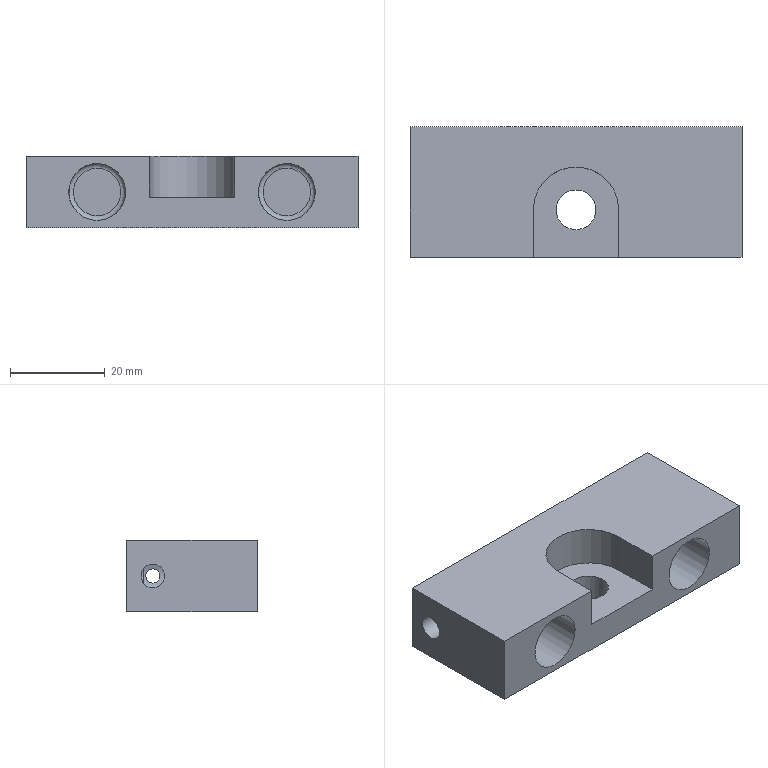NC program | NX | posted with a generic post | part box 70 x 27.5 x 15 mm
Lines 28 to 859 of 3781:
(PLANAR_MILL_8 , TOOL : D8-25-D8-60-3T-ROUGH)
N48 T03 M6
N50 G54
N52 G17 G0 G90 X-21.509 Y1.151 B0. C0. S2500 M3
N54 G43 Z20. H3
N56 Z1. B-180. C-180.
N58 G94 G1 X-21.592 Y1.043 Z0.993 F600.
N60 X-21.699 Y0.857 Z0.982
N62 X-21.809 Y0.59 Z0.966
N64 X-21.878 Y0.308 Z0.951
N66 X-21.903 Y0.019 Z0.936
N68 X-21.884 Y-0.27 Z0.921
N70 X-21.821 Y-0.553 Z0.906
N72 X-21.716 Y-0.823 Z0.891
N74 X-21.571 Y-1.074 Z0.875
N76 X-21.389 Y-1.3 Z0.86
N78 X-21.176 Y-1.496 Z0.845
N80 X-20.935 Y-1.658 Z0.83
N82 X-20.672 Y-1.78 Z0.815
N84 X-20.394 Y-1.862 Z0.799
N86 X-20.107 Y-1.9 Z0.784
N88 X-19.893 Z0.773
N90 X-19.606 Y-1.862 Z0.758
N92 X-19.328 Y-1.78 Z0.743
N94 X-19.065 Y-1.658 Z0.727
N96 X-18.824 Y-1.496 Z0.712
N98 X-18.611 Y-1.3 Z0.697
N100 X-18.429 Y-1.074 Z0.682
N102 X-18.284 Y-0.823 Z0.667
N104 X-18.179 Y-0.553 Z0.651
N106 X-18.116 Y-0.27 Z0.636
N108 X-18.097 Y0.019 Z0.621
N110 X-18.122 Y0.308 Z0.606
N112 X-18.191 Y0.59 Z0.591
N114 X-18.301 Y0.857 Z0.575
N116 X-18.408 Y1.043 Z0.564
N118 X-18.589 Y1.277 Z0.549
N120 X-18.804 Y1.48 Z0.533
N122 X-19.049 Y1.648 Z0.518
N124 X-19.316 Y1.776 Z0.502
N126 X-19.6 Y1.86 Z0.487
N128 X-19.893 Y1.9 Z0.471
N130 X-20.107 Z0.46
N132 X-20.4 Y1.86 Z0.444
N134 X-20.684 Y1.776 Z0.429
N136 X-20.952 Y1.648 Z0.413
N138 X-21.196 Y1.48 Z0.398
N140 X-21.411 Y1.277 Z0.382
N142 X-21.592 Y1.043 Z0.367
N144 X-21.699 Y0.857 Z0.356
N146 X-21.809 Y0.59 Z0.34
N148 X-21.878 Y0.308 Z0.325
N150 X-21.903 Y0.019 Z0.31
N152 X-21.884 Y-0.27 Z0.295
N154 X-21.821 Y-0.553 Z0.28
N156 X-21.716 Y-0.823 Z0.264
N158 X-21.571 Y-1.074 Z0.249
N160 X-21.389 Y-1.3 Z0.234
N162 X-21.176 Y-1.496 Z0.219
N164 X-20.935 Y-1.658 Z0.204
N166 X-20.672 Y-1.78 Z0.189
N168 X-20.394 Y-1.862 Z0.173
N170 X-20.107 Y-1.9 Z0.158
N172 X-19.893 Z0.147
N174 X-19.606 Y-1.862 Z0.132
N176 X-19.328 Y-1.78 Z0.117
N178 X-19.065 Y-1.658 Z0.101
N180 X-18.824 Y-1.496 Z0.086
N182 X-18.611 Y-1.3 Z0.071
N184 X-18.429 Y-1.074 Z0.056
N186 X-18.284 Y-0.823 Z0.041
N188 X-18.179 Y-0.553 Z0.025
N190 X-18.116 Y-0.27 Z0.01
N192 X-18.097 Y0.019 Z-0.005
N194 X-18.122 Y0.308 Z-0.02
N196 X-18.191 Y0.59 Z-0.035
N198 X-18.301 Y0.857 Z-0.051
N200 X-18.408 Y1.043 Z-0.062
N202 X-18.589 Y1.277 Z-0.077
N204 X-18.804 Y1.48 Z-0.093
N206 X-19.049 Y1.648 Z-0.108
N208 X-19.316 Y1.776 Z-0.124
N210 X-19.6 Y1.86 Z-0.139
N212 X-19.893 Y1.9 Z-0.155
N214 X-20.107 Z-0.166
N216 X-20.4 Y1.86 Z-0.182
N218 X-20.684 Y1.776 Z-0.197
N220 X-20.952 Y1.648 Z-0.213
N222 X-21.196 Y1.48 Z-0.228
N224 X-21.411 Y1.277 Z-0.244
N226 X-21.592 Y1.043 Z-0.259
N228 X-21.699 Y0.857 Z-0.27
N230 X-21.809 Y0.59 Z-0.286
N232 X-21.878 Y0.308 Z-0.301
N234 X-21.903 Y0.019 Z-0.316
N236 X-21.884 Y-0.27 Z-0.331
N238 X-21.821 Y-0.553 Z-0.346
N240 X-21.716 Y-0.823 Z-0.362
N242 X-21.571 Y-1.074 Z-0.377
N244 X-21.389 Y-1.3 Z-0.392
N246 X-21.176 Y-1.496 Z-0.407
N248 X-20.935 Y-1.658 Z-0.422
N250 X-20.672 Y-1.78 Z-0.438
N252 X-20.394 Y-1.862 Z-0.453
N254 X-20.107 Y-1.9 Z-0.468
N256 X-19.893 Z-0.479
N258 X-19.606 Y-1.862 Z-0.494
N260 X-19.328 Y-1.78 Z-0.509
N262 X-19.065 Y-1.658 Z-0.525
N264 X-18.824 Y-1.496 Z-0.54
N266 X-18.611 Y-1.3 Z-0.555
N268 X-18.429 Y-1.074 Z-0.57
N270 X-18.284 Y-0.823 Z-0.585
N272 X-18.179 Y-0.553 Z-0.601
N274 X-18.116 Y-0.27 Z-0.616
N276 X-18.097 Y0.019 Z-0.631
N278 X-18.122 Y0.308 Z-0.646
N280 X-18.191 Y0.59 Z-0.661
N282 X-18.301 Y0.857 Z-0.677
N284 X-18.408 Y1.043 Z-0.688
N286 X-18.589 Y1.277 Z-0.703
N288 X-18.804 Y1.48 Z-0.719
N290 X-19.049 Y1.648 Z-0.734
N292 X-19.316 Y1.776 Z-0.75
N294 X-19.6 Y1.86 Z-0.765
N296 X-19.893 Y1.9 Z-0.781
N298 X-20.107 Z-0.792
N300 X-20.4 Y1.86 Z-0.808
N302 X-20.684 Y1.776 Z-0.823
N304 X-20.952 Y1.648 Z-0.839
N306 X-21.196 Y1.48 Z-0.854
N308 X-21.411 Y1.277 Z-0.87
N310 X-21.592 Y1.043 Z-0.885
N312 X-21.699 Y0.857 Z-0.896
N314 X-21.809 Y0.59 Z-0.912
N316 X-21.878 Y0.308 Z-0.927
N318 X-21.903 Y0.019 Z-0.942
N320 X-21.884 Y-0.27 Z-0.957
N322 X-21.821 Y-0.553 Z-0.972
N324 X-21.716 Y-0.823 Z-0.988
N326 X-21.571 Y-1.074 Z-1.003
N328 X-21.389 Y-1.3 Z-1.018
N330 X-21.176 Y-1.496 Z-1.033
N332 X-20.935 Y-1.658 Z-1.048
N334 X-20.672 Y-1.78 Z-1.064
N336 X-20.394 Y-1.862 Z-1.079
N338 X-20.107 Y-1.9 Z-1.094
N340 X-19.893 Z-1.105
N342 X-19.606 Y-1.862 Z-1.12
N344 X-19.328 Y-1.78 Z-1.136
N346 X-19.065 Y-1.658 Z-1.151
N348 X-18.824 Y-1.496 Z-1.166
N350 X-18.611 Y-1.3 Z-1.181
N352 X-18.429 Y-1.074 Z-1.196
N354 X-18.284 Y-0.823 Z-1.211
N356 X-18.179 Y-0.553 Z-1.227
N358 X-18.116 Y-0.27 Z-1.242
N360 X-18.097 Y0.019 Z-1.257
N362 X-18.122 Y0.308 Z-1.272
N364 X-18.191 Y0.59 Z-1.287
N366 X-18.301 Y0.857 Z-1.303
N368 X-18.408 Y1.043 Z-1.314
N370 X-18.589 Y1.277 Z-1.329
N372 X-18.804 Y1.48 Z-1.345
N374 X-19.049 Y1.648 Z-1.36
N376 X-19.316 Y1.776 Z-1.376
N378 X-19.6 Y1.86 Z-1.391
N380 X-19.893 Y1.9 Z-1.407
N382 X-20.107 Z-1.418
N384 X-20.4 Y1.86 Z-1.434
N386 X-20.684 Y1.776 Z-1.449
N388 X-20.952 Y1.648 Z-1.465
N390 X-21.196 Y1.48 Z-1.48
N392 X-21.411 Y1.277 Z-1.496
N394 X-21.592 Y1.043 Z-1.511
N396 X-21.699 Y0.857 Z-1.523
N398 X-21.809 Y0.59 Z-1.538
N400 X-21.878 Y0.308 Z-1.553
N402 X-21.903 Y0.019 Z-1.568
N404 X-21.884 Y-0.27 Z-1.583
N406 X-21.821 Y-0.553 Z-1.598
N408 X-21.716 Y-0.823 Z-1.614
N410 X-21.571 Y-1.074 Z-1.629
N412 X-21.389 Y-1.3 Z-1.644
N414 X-21.176 Y-1.496 Z-1.659
N416 X-20.935 Y-1.658 Z-1.674
N418 X-20.672 Y-1.78 Z-1.69
N420 X-20.394 Y-1.862 Z-1.705
N422 X-20.107 Y-1.9 Z-1.72
N424 X-19.893 Z-1.731
N426 X-19.606 Y-1.862 Z-1.746
N428 X-19.328 Y-1.78 Z-1.762
N430 X-19.065 Y-1.658 Z-1.777
N432 X-18.824 Y-1.496 Z-1.792
N434 X-18.611 Y-1.3 Z-1.807
N436 X-18.429 Y-1.074 Z-1.822
N438 X-18.284 Y-0.823 Z-1.838
N440 X-18.179 Y-0.553 Z-1.853
N442 X-18.116 Y-0.27 Z-1.868
N444 X-18.097 Y0.019 Z-1.883
N446 X-18.122 Y0.308 Z-1.898
N448 X-18.191 Y0.59 Z-1.913
N450 X-18.301 Y0.857 Z-1.929
N452 X-18.408 Y1.043 Z-1.94
N454 X-18.589 Y1.277 Z-1.955
N456 X-18.804 Y1.48 Z-1.971
N458 X-19.049 Y1.648 Z-1.986
N460 X-19.316 Y1.776 Z-2.002
N462 X-19.6 Y1.86 Z-2.017
N464 X-19.893 Y1.9 Z-2.033
N466 X-20.107 Z-2.044
N468 X-20.4 Y1.86 Z-2.06
N470 X-20.684 Y1.776 Z-2.075
N472 X-20.952 Y1.648 Z-2.091
N474 X-21.196 Y1.48 Z-2.106
N476 X-21.411 Y1.277 Z-2.122
N478 X-21.592 Y1.043 Z-2.137
N480 X-21.699 Y0.857 Z-2.149
N482 X-21.809 Y0.59 Z-2.164
N484 X-21.878 Y0.308 Z-2.179
N486 X-21.903 Y0.019 Z-2.194
N488 X-21.884 Y-0.27 Z-2.209
N490 X-21.821 Y-0.553 Z-2.225
N492 X-21.716 Y-0.823 Z-2.24
N494 X-21.571 Y-1.074 Z-2.255
N496 X-21.389 Y-1.3 Z-2.27
N498 X-21.176 Y-1.496 Z-2.285
N500 X-20.935 Y-1.658 Z-2.3
N502 X-20.672 Y-1.78 Z-2.316
N504 X-20.394 Y-1.862 Z-2.331
N506 X-20.107 Y-1.9 Z-2.346
N508 X-19.893 Z-2.357
N510 X-19.606 Y-1.862 Z-2.372
N512 X-19.328 Y-1.78 Z-2.388
N514 X-19.065 Y-1.658 Z-2.403
N516 X-18.824 Y-1.496 Z-2.418
N518 X-18.611 Y-1.3 Z-2.433
N520 X-18.429 Y-1.074 Z-2.448
N522 X-18.284 Y-0.823 Z-2.464
N524 X-18.179 Y-0.553 Z-2.479
N526 X-18.116 Y-0.27 Z-2.494
N528 X-18.097 Y0.019 Z-2.509
N530 X-18.122 Y0.308 Z-2.524
N532 X-18.191 Y0.59 Z-2.54
N534 X-18.301 Y0.857 Z-2.555
N536 X-18.408 Y1.043 Z-2.566
N538 X-18.589 Y1.277 Z-2.581
N540 X-18.804 Y1.48 Z-2.597
N542 X-19.049 Y1.648 Z-2.612
N544 X-19.316 Y1.776 Z-2.628
N546 X-19.6 Y1.86 Z-2.644
N548 X-19.893 Y1.9 Z-2.659
N550 X-20.107 Z-2.67
N552 X-20.4 Y1.86 Z-2.686
N554 X-20.684 Y1.776 Z-2.701
N556 X-20.952 Y1.648 Z-2.717
N558 X-21.196 Y1.48 Z-2.732
N560 X-21.411 Y1.277 Z-2.748
N562 X-21.592 Y1.043 Z-2.763
N564 X-21.699 Y0.857 Z-2.775
N566 X-21.809 Y0.59 Z-2.79
N568 X-21.878 Y0.308 Z-2.805
N570 X-21.903 Y0.019 Z-2.82
N572 X-21.884 Y-0.27 Z-2.835
N574 X-21.821 Y-0.553 Z-2.851
N576 X-21.716 Y-0.823 Z-2.866
N578 X-21.571 Y-1.074 Z-2.881
N580 X-21.389 Y-1.3 Z-2.896
N582 X-21.176 Y-1.496 Z-2.911
N584 X-20.935 Y-1.658 Z-2.926
N586 X-20.672 Y-1.78 Z-2.942
N588 X-20.394 Y-1.862 Z-2.957
N590 X-20.107 Y-1.9 Z-2.972
N592 X-19.893 Z-2.983
N594 X-19.606 Y-1.862 Z-2.998
N596 X-19.328 Y-1.78 Z-3.014
N598 X-19.065 Y-1.658 Z-3.029
N600 X-18.824 Y-1.496 Z-3.044
N602 X-18.611 Y-1.3 Z-3.059
N604 X-18.429 Y-1.074 Z-3.074
N606 X-18.284 Y-0.823 Z-3.09
N608 X-18.179 Y-0.553 Z-3.105
N610 X-18.116 Y-0.27 Z-3.12
N612 X-18.097 Y0.019 Z-3.135
N614 X-18.122 Y0.308 Z-3.15
N616 X-18.191 Y0.59 Z-3.166
N618 X-18.301 Y0.857 Z-3.181
N620 X-18.408 Y1.043 Z-3.192
N622 X-18.589 Y1.277 Z-3.207
N624 X-18.804 Y1.48 Z-3.223
N626 X-19.049 Y1.648 Z-3.239
N628 X-19.316 Y1.776 Z-3.254
N630 X-19.6 Y1.86 Z-3.27
N632 X-19.893 Y1.9 Z-3.285
N634 X-20.107 Z-3.296
N636 X-20.4 Y1.86 Z-3.312
N638 X-20.684 Y1.776 Z-3.327
N640 X-20.952 Y1.648 Z-3.343
N642 X-21.196 Y1.48 Z-3.358
N644 X-21.411 Y1.277 Z-3.374
N646 X-21.592 Y1.043 Z-3.389
N648 X-21.699 Y0.857 Z-3.401
N650 X-21.809 Y0.59 Z-3.416
N652 X-21.878 Y0.308 Z-3.431
N654 X-21.903 Y0.019 Z-3.446
N656 X-21.884 Y-0.27 Z-3.461
N658 X-21.821 Y-0.553 Z-3.477
N660 X-21.716 Y-0.823 Z-3.492
N662 X-21.571 Y-1.074 Z-3.507
N664 X-21.389 Y-1.3 Z-3.522
N666 X-21.176 Y-1.496 Z-3.537
N668 X-20.935 Y-1.658 Z-3.553
N670 X-20.672 Y-1.78 Z-3.568
N672 X-20.394 Y-1.862 Z-3.583
N674 X-20.107 Y-1.9 Z-3.598
N676 X-19.893 Z-3.609
N678 X-19.606 Y-1.862 Z-3.624
N680 X-19.328 Y-1.78 Z-3.64
N682 X-19.065 Y-1.658 Z-3.655
N684 X-18.824 Y-1.496 Z-3.67
N686 X-18.611 Y-1.3 Z-3.685
N688 X-18.429 Y-1.074 Z-3.7
N690 X-18.284 Y-0.823 Z-3.716
N692 X-18.179 Y-0.553 Z-3.731
N694 X-18.116 Y-0.27 Z-3.746
N696 X-18.097 Y0.019 Z-3.761
N698 X-18.122 Y0.308 Z-3.776
N700 X-18.191 Y0.59 Z-3.792
N702 X-18.301 Y0.857 Z-3.807
N704 X-18.408 Y1.043 Z-3.818
N706 X-18.589 Y1.277 Z-3.834
N708 X-18.804 Y1.48 Z-3.849
N710 X-19.049 Y1.648 Z-3.865
N712 X-19.316 Y1.776 Z-3.88
N714 X-19.6 Y1.86 Z-3.896
N716 X-19.893 Y1.9 Z-3.911
N718 X-20.107 Z-3.922
N720 X-20.4 Y1.86 Z-3.938
N722 X-20.684 Y1.776 Z-3.953
N724 X-20.952 Y1.648 Z-3.969
N726 X-21.196 Y1.48 Z-3.984
N728 X-21.411 Y1.277 Z-4.
N730 X-21.592 Y1.043 Z-4.015
N732 X-21.699 Y0.857 Z-4.027
N734 X-21.809 Y0.59 Z-4.042
N736 X-21.878 Y0.308 Z-4.057
N738 X-21.903 Y0.019 Z-4.072
N740 X-21.884 Y-0.27 Z-4.087
N742 X-21.821 Y-0.553 Z-4.103
N744 X-21.716 Y-0.823 Z-4.118
N746 X-21.571 Y-1.074 Z-4.133
N748 X-21.389 Y-1.3 Z-4.148
N750 X-21.176 Y-1.496 Z-4.163
N752 X-20.935 Y-1.658 Z-4.179
N754 X-20.672 Y-1.78 Z-4.194
N756 X-20.394 Y-1.862 Z-4.209
N758 X-20.107 Y-1.9 Z-4.224
N760 X-19.893 Z-4.235
N762 X-19.606 Y-1.862 Z-4.251
N764 X-19.328 Y-1.78 Z-4.266
N766 X-19.065 Y-1.658 Z-4.281
N768 X-18.824 Y-1.496 Z-4.296
N770 X-18.611 Y-1.3 Z-4.311
N772 X-18.429 Y-1.074 Z-4.326
N774 X-18.284 Y-0.823 Z-4.342
N776 X-18.179 Y-0.553 Z-4.357
N778 X-18.116 Y-0.27 Z-4.372
N780 X-18.097 Y0.019 Z-4.387
N782 X-18.122 Y0.308 Z-4.402
N784 X-18.191 Y0.59 Z-4.418
N786 X-18.301 Y0.857 Z-4.433
N788 X-18.408 Y1.043 Z-4.444
N790 X-18.589 Y1.277 Z-4.46
N792 X-18.804 Y1.48 Z-4.475
N794 X-19.049 Y1.648 Z-4.491
N796 X-19.316 Y1.776 Z-4.506
N798 X-19.6 Y1.86 Z-4.522
N800 X-19.893 Y1.9 Z-4.537
N802 X-20.107 Z-4.548
N804 X-20.4 Y1.86 Z-4.564
N806 X-20.684 Y1.776 Z-4.579
N808 X-20.952 Y1.648 Z-4.595
N810 X-21.196 Y1.48 Z-4.61
N812 X-21.411 Y1.277 Z-4.626
N814 X-21.592 Y1.043 Z-4.642
N816 X-21.699 Y0.857 Z-4.653
N818 X-21.809 Y0.59 Z-4.668
N820 X-21.878 Y0.308 Z-4.683
N822 X-21.903 Y0.019 Z-4.698
N824 X-21.884 Y-0.27 Z-4.713
N826 X-21.821 Y-0.553 Z-4.729
N828 X-21.716 Y-0.823 Z-4.744
N830 X-21.571 Y-1.074 Z-4.759
N832 X-21.389 Y-1.3 Z-4.774
N834 X-21.176 Y-1.496 Z-4.789
N836 X-20.935 Y-1.658 Z-4.805
N838 X-20.672 Y-1.78 Z-4.82
N840 X-20.394 Y-1.862 Z-4.835
N842 X-20.107 Y-1.9 Z-4.85
N844 X-19.893 Z-4.861
N846 X-19.606 Y-1.862 Z-4.877
N848 X-19.328 Y-1.78 Z-4.892
N850 X-19.065 Y-1.658 Z-4.907
N852 X-18.824 Y-1.496 Z-4.922
N854 X-18.611 Y-1.3 Z-4.937
N856 X-18.429 Y-1.074 Z-4.953
N858 X-18.284 Y-0.823 Z-4.968
N860 X-18.179 Y-0.553 Z-4.983
N862 X-18.116 Y-0.27 Z-4.998
N864 X-18.097 Y0.019 Z-5.013
N866 X-18.122 Y0.308 Z-5.028
N868 X-18.191 Y0.59 Z-5.044
N870 X-18.301 Y0.857 Z-5.059
N872 X-18.408 Y1.043 Z-5.07
N874 X-18.589 Y1.277 Z-5.086
N876 X-18.804 Y1.48 Z-5.101
N878 X-19.049 Y1.648 Z-5.117
N880 X-19.316 Y1.776 Z-5.132
N882 X-19.6 Y1.86 Z-5.148
N884 X-19.893 Y1.9 Z-5.163
N886 X-20.107 Z-5.174
N888 X-20.4 Y1.86 Z-5.19
N890 X-20.684 Y1.776 Z-5.205
N892 X-20.952 Y1.648 Z-5.221
N894 X-21.196 Y1.48 Z-5.237
N896 X-21.411 Y1.277 Z-5.252
N898 X-21.592 Y1.043 Z-5.268
N900 X-21.699 Y0.857 Z-5.279
N902 X-21.809 Y0.59 Z-5.294
N904 X-21.878 Y0.308 Z-5.309
N906 X-21.903 Y0.019 Z-5.324
N908 X-21.884 Y-0.27 Z-5.34
N910 X-21.821 Y-0.553 Z-5.355
N912 X-21.716 Y-0.823 Z-5.37
N914 X-21.571 Y-1.074 Z-5.385
N916 X-21.389 Y-1.3 Z-5.4
N918 X-21.176 Y-1.496 Z-5.415
N920 X-20.935 Y-1.658 Z-5.431
N922 X-20.672 Y-1.78 Z-5.446
N924 X-20.394 Y-1.862 Z-5.461
N926 X-20.107 Y-1.9 Z-5.476
N928 X-19.893 Z-5.487
N930 X-19.606 Y-1.862 Z-5.503
N932 X-19.328 Y-1.78 Z-5.518
N934 X-19.065 Y-1.658 Z-5.533
N936 X-18.824 Y-1.496 Z-5.548
N938 X-18.611 Y-1.3 Z-5.563
N940 X-18.429 Y-1.074 Z-5.579
N942 X-18.284 Y-0.823 Z-5.594
N944 X-18.179 Y-0.553 Z-5.609
N946 X-18.116 Y-0.27 Z-5.624
N948 X-18.097 Y0.019 Z-5.639
N950 X-18.122 Y0.308 Z-5.655
N952 X-18.191 Y0.59 Z-5.67
N954 X-18.301 Y0.857 Z-5.685
N956 X-18.408 Y1.043 Z-5.696
N958 X-18.589 Y1.277 Z-5.712
N960 X-18.804 Y1.48 Z-5.727
N962 X-19.049 Y1.648 Z-5.743
N964 X-19.316 Y1.776 Z-5.758
N966 X-19.6 Y1.86 Z-5.774
N968 X-19.893 Y1.9 Z-5.789
N970 X-20.107 Z-5.8
N972 X-20.4 Y1.86 Z-5.816
N974 X-20.684 Y1.776 Z-5.831
N976 X-20.952 Y1.648 Z-5.847
N978 X-21.196 Y1.48 Z-5.863
N980 X-21.411 Y1.277 Z-5.878
N982 X-21.592 Y1.043 Z-5.894
N984 X-21.699 Y0.857 Z-5.905
N986 X-21.809 Y0.59 Z-5.92
N988 X-21.878 Y0.308 Z-5.935
N990 X-21.903 Y0.019 Z-5.95
N992 X-21.884 Y-0.27 Z-5.966
N994 X-21.821 Y-0.553 Z-5.981
N996 X-21.716 Y-0.823 Z-5.996
N998 X-21.571 Y-1.074 Z-6.011
N1000 X-21.389 Y-1.3 Z-6.026
N1002 X-21.176 Y-1.496 Z-6.042
N1004 X-20.935 Y-1.658 Z-6.057
N1006 X-20.672 Y-1.78 Z-6.072
N1008 X-20.394 Y-1.862 Z-6.087
N1010 X-20.107 Y-1.9 Z-6.102
N1012 X-19.893 Z-6.113
N1014 X-19.606 Y-1.862 Z-6.129
N1016 X-19.328 Y-1.78 Z-6.144
N1018 X-19.065 Y-1.658 Z-6.159
N1020 X-18.824 Y-1.496 Z-6.174
N1022 X-18.611 Y-1.3 Z-6.189
N1024 X-18.429 Y-1.074 Z-6.205
N1026 X-18.284 Y-0.823 Z-6.22
N1028 X-18.179 Y-0.553 Z-6.235
N1030 X-18.116 Y-0.27 Z-6.25
N1032 X-18.097 Y0.019 Z-6.265
N1034 X-18.122 Y0.308 Z-6.281
N1036 X-18.191 Y0.59 Z-6.296
N1038 X-18.301 Y0.857 Z-6.311
N1040 X-18.408 Y1.043 Z-6.322
N1042 X-18.589 Y1.277 Z-6.338
N1044 X-18.804 Y1.48 Z-6.353
N1046 X-19.049 Y1.648 Z-6.369
N1048 X-19.316 Y1.776 Z-6.384
N1050 X-19.6 Y1.86 Z-6.4
N1052 X-19.893 Y1.9 Z-6.415
N1054 X-20.107 Z-6.426
N1056 X-20.4 Y1.86 Z-6.442
N1058 X-20.684 Y1.776 Z-6.458
N1060 X-20.952 Y1.648 Z-6.473
N1062 X-21.196 Y1.48 Z-6.489
N1064 X-21.411 Y1.277 Z-6.504
N1066 X-21.592 Y1.043 Z-6.52
N1068 X-21.699 Y0.857 Z-6.531
N1070 X-21.809 Y0.59 Z-6.546
N1072 X-21.878 Y0.308 Z-6.561
N1074 X-21.903 Y0.019 Z-6.576
N1076 X-21.884 Y-0.27 Z-6.592
N1078 X-21.821 Y-0.553 Z-6.607
N1080 X-21.716 Y-0.823 Z-6.622
N1082 X-21.571 Y-1.074 Z-6.637
N1084 X-21.389 Y-1.3 Z-6.652
N1086 X-21.176 Y-1.496 Z-6.668
N1088 X-20.935 Y-1.658 Z-6.683
N1090 X-20.672 Y-1.78 Z-6.698
N1092 X-20.394 Y-1.862 Z-6.713
N1094 X-20.107 Y-1.9 Z-6.728
N1096 X-19.893 Z-6.74
N1098 X-19.606 Y-1.862 Z-6.755
N1100 X-19.328 Y-1.78 Z-6.77
N1102 X-19.065 Y-1.658 Z-6.785
N1104 X-18.824 Y-1.496 Z-6.8
N1106 X-18.611 Y-1.3 Z-6.815
N1108 X-18.429 Y-1.074 Z-6.831
N1110 X-18.284 Y-0.823 Z-6.846
N1112 X-18.179 Y-0.553 Z-6.861
N1114 X-18.116 Y-0.27 Z-6.876
N1116 X-18.097 Y0.019 Z-6.891
N1118 X-18.122 Y0.308 Z-6.907
N1120 X-18.191 Y0.59 Z-6.922
N1122 X-18.301 Y0.857 Z-6.937
N1124 X-18.408 Y1.043 Z-6.948
N1126 X-18.589 Y1.277 Z-6.964
N1128 X-18.804 Y1.48 Z-6.979
N1130 X-19.049 Y1.648 Z-6.995
N1132 X-19.316 Y1.776 Z-7.01
N1134 X-19.6 Y1.86 Z-7.026
N1136 X-19.893 Y1.9 Z-7.041
N1138 X-20.107 Z-7.053
N1140 X-20.4 Y1.86 Z-7.068
N1142 X-20.684 Y1.776 Z-7.084
N1144 X-20.952 Y1.648 Z-7.099
N1146 X-21.196 Y1.48 Z-7.115
N1148 X-21.411 Y1.277 Z-7.13
N1150 X-21.592 Y1.043 Z-7.146
N1152 X-21.699 Y0.857 Z-7.157
N1154 X-21.809 Y0.59 Z-7.172
N1156 X-21.878 Y0.308 Z-7.187
N1158 X-21.903 Y0.019 Z-7.202
N1160 X-21.884 Y-0.27 Z-7.218
N1162 X-21.821 Y-0.553 Z-7.233
N1164 X-21.716 Y-0.823 Z-7.248
N1166 X-21.571 Y-1.074 Z-7.263
N1168 X-21.389 Y-1.3 Z-7.278
N1170 X-21.176 Y-1.496 Z-7.294
N1172 X-20.935 Y-1.658 Z-7.309
N1174 X-20.672 Y-1.78 Z-7.324
N1176 X-20.394 Y-1.862 Z-7.339
N1178 X-20.107 Y-1.9 Z-7.354
N1180 X-19.893 Z-7.366
N1182 X-19.606 Y-1.862 Z-7.381
N1184 X-19.328 Y-1.78 Z-7.396
N1186 X-19.065 Y-1.658 Z-7.411
N1188 X-18.824 Y-1.496 Z-7.426
N1190 X-18.611 Y-1.3 Z-7.442
N1192 X-18.429 Y-1.074 Z-7.457
N1194 X-18.284 Y-0.823 Z-7.472
N1196 X-18.179 Y-0.553 Z-7.487
N1198 X-18.116 Y-0.27 Z-7.502
N1200 X-18.097 Y0.019 Z-7.517
N1202 X-18.122 Y0.308 Z-7.533
N1204 X-18.191 Y0.59 Z-7.548
N1206 X-18.301 Y0.857 Z-7.563
N1208 X-18.408 Y1.043 Z-7.574
N1210 X-18.589 Y1.277 Z-7.59
N1212 X-18.804 Y1.48 Z-7.605
N1214 X-19.049 Y1.648 Z-7.621
N1216 X-19.316 Y1.776 Z-7.636
N1218 X-19.6 Y1.86 Z-7.652
N1220 X-19.893 Y1.9 Z-7.667
N1222 X-20.107 Z-7.679
N1224 X-20.4 Y1.86 Z-7.694
N1226 X-20.684 Y1.776 Z-7.71
N1228 X-20.952 Y1.648 Z-7.725
N1230 X-21.196 Y1.48 Z-7.741
N1232 X-21.411 Y1.277 Z-7.756
N1234 X-21.592 Y1.043 Z-7.772
N1236 X-21.699 Y0.857 Z-7.783
N1238 X-21.809 Y0.59 Z-7.798
N1240 X-21.878 Y0.308 Z-7.813
N1242 X-21.903 Y0.019 Z-7.828
N1244 X-21.884 Y-0.27 Z-7.844
N1246 X-21.821 Y-0.553 Z-7.859
N1248 X-21.716 Y-0.823 Z-7.874
N1250 X-21.571 Y-1.074 Z-7.889
N1252 X-21.389 Y-1.3 Z-7.904
N1254 X-21.176 Y-1.496 Z-7.92
N1256 X-20.935 Y-1.658 Z-7.935
N1258 X-20.672 Y-1.78 Z-7.95
N1260 X-20.394 Y-1.862 Z-7.965
N1262 X-20.107 Y-1.9 Z-7.98
N1264 X-19.893 Z-7.992
N1266 X-19.606 Y-1.862 Z-8.007
N1268 X-19.328 Y-1.78 Z-8.022
N1270 X-19.065 Y-1.658 Z-8.037
N1272 X-18.824 Y-1.496 Z-8.052
N1274 X-18.611 Y-1.3 Z-8.068
N1276 X-18.429 Y-1.074 Z-8.083
N1278 X-18.284 Y-0.823 Z-8.098
N1280 X-18.179 Y-0.553 Z-8.113
N1282 X-18.116 Y-0.27 Z-8.128
N1284 X-18.097 Y0.019 Z-8.143
N1286 X-18.122 Y0.308 Z-8.159
N1288 X-18.191 Y0.59 Z-8.174
N1290 X-18.301 Y0.857 Z-8.189
N1292 X-18.408 Y1.043 Z-8.2
N1294 X-18.589 Y1.277 Z-8.216
N1296 X-18.804 Y1.48 Z-8.231
N1298 X-19.049 Y1.648 Z-8.247
N1300 X-19.316 Y1.776 Z-8.262
N1302 X-19.6 Y1.86 Z-8.278
N1304 X-19.893 Y1.9 Z-8.293
N1306 X-20.107 Z-8.305
N1308 X-20.4 Y1.86 Z-8.32
N1310 X-20.684 Y1.776 Z-8.336
N1312 X-20.952 Y1.648 Z-8.351
N1314 X-21.196 Y1.48 Z-8.367
N1316 X-21.411 Y1.277 Z-8.382
N1318 X-21.592 Y1.043 Z-8.398
N1320 X-21.699 Y0.857 Z-8.409
N1322 X-21.809 Y0.59 Z-8.424
N1324 X-21.878 Y0.308 Z-8.439
N1326 X-21.903 Y0.019 Z-8.455
N1328 X-21.884 Y-0.27 Z-8.47
N1330 X-21.821 Y-0.553 Z-8.485
N1332 X-21.716 Y-0.823 Z-8.5
N1334 X-21.571 Y-1.074 Z-8.515
N1336 X-21.389 Y-1.3 Z-8.53
N1338 X-21.176 Y-1.496 Z-8.546
N1340 X-20.935 Y-1.658 Z-8.561
N1342 X-20.672 Y-1.78 Z-8.576
N1344 X-20.394 Y-1.862 Z-8.591
N1346 X-20.107 Y-1.9 Z-8.606
N1348 X-19.893 Z-8.618
N1350 X-19.606 Y-1.862 Z-8.633
N1352 X-19.328 Y-1.78 Z-8.648
N1354 X-19.065 Y-1.658 Z-8.663
N1356 X-18.824 Y-1.496 Z-8.678
N1358 X-18.611 Y-1.3 Z-8.694
N1360 X-18.429 Y-1.074 Z-8.709
N1362 X-18.284 Y-0.823 Z-8.724
N1364 X-18.179 Y-0.553 Z-8.739
N1366 X-18.116 Y-0.27 Z-8.754
N1368 X-18.097 Y0.019 Z-8.77
N1370 X-18.122 Y0.308 Z-8.785
N1372 X-18.191 Y0.59 Z-8.8
N1374 X-18.301 Y0.857 Z-8.815
N1376 X-18.408 Y1.043 Z-8.826
N1378 X-18.589 Y1.277 Z-8.842
N1380 X-18.804 Y1.48 Z-8.857
N1382 X-19.049 Y1.648 Z-8.873
N1384 X-19.316 Y1.776 Z-8.888
N1386 X-19.6 Y1.86 Z-8.904
N1388 X-19.893 Y1.9 Z-8.919
N1390 X-20.107 Z-8.931
N1392 X-20.4 Y1.86 Z-8.946
N1394 X-20.684 Y1.776 Z-8.962
N1396 X-20.952 Y1.648 Z-8.977
N1398 X-21.196 Y1.48 Z-8.993
N1400 X-21.411 Y1.277 Z-9.008
N1402 X-21.592 Y1.043 Z-9.024
N1404 X-21.699 Y0.857 Z-9.035
N1406 X-21.809 Y0.59 Z-9.05
N1408 X-21.878 Y0.308 Z-9.065
N1410 X-21.903 Y0.019 Z-9.081
N1412 X-21.884 Y-0.27 Z-9.096
N1414 X-21.821 Y-0.553 Z-9.111
N1416 X-21.716 Y-0.823 Z-9.126
N1418 X-21.571 Y-1.074 Z-9.141
N1420 X-21.389 Y-1.3 Z-9.157
N1422 X-21.176 Y-1.496 Z-9.172
N1424 X-20.935 Y-1.658 Z-9.187
N1426 X-20.672 Y-1.78 Z-9.202
N1428 X-20.394 Y-1.862 Z-9.217
N1430 X-20.107 Y-1.9 Z-9.232
N1432 X-19.893 Z-9.244
N1434 X-19.606 Y-1.862 Z-9.259
N1436 X-19.328 Y-1.78 Z-9.274
N1438 X-19.065 Y-1.658 Z-9.289
N1440 X-18.824 Y-1.496 Z-9.304
N1442 X-18.611 Y-1.3 Z-9.32
N1444 X-18.429 Y-1.074 Z-9.335
N1446 X-18.284 Y-0.823 Z-9.35
N1448 X-18.179 Y-0.553 Z-9.365
N1450 X-18.116 Y-0.27 Z-9.38
N1452 X-18.097 Y0.019 Z-9.396
N1454 X-18.122 Y0.308 Z-9.411
N1456 X-18.191 Y0.59 Z-9.426
N1458 X-18.301 Y0.857 Z-9.441
N1460 X-18.408 Y1.043 Z-9.452
N1462 X-18.589 Y1.277 Z-9.468
N1464 X-18.804 Y1.48 Z-9.483
N1466 X-19.049 Y1.648 Z-9.499
N1468 X-19.316 Y1.776 Z-9.514
N1470 X-19.6 Y1.86 Z-9.53
N1472 X-19.893 Y1.9 Z-9.545
N1474 X-20.107 Z-9.557
N1476 X-20.4 Y1.86 Z-9.572
N1478 X-20.684 Y1.776 Z-9.588
N1480 X-20.952 Y1.648 Z-9.603
N1482 X-21.196 Y1.48 Z-9.619
N1484 X-21.411 Y1.277 Z-9.634
N1486 X-21.592 Y1.043 Z-9.65
N1488 X-21.699 Y0.857 Z-9.661
N1490 X-21.809 Y0.59 Z-9.676
N1492 X-21.878 Y0.308 Z-9.691
N1494 X-21.903 Y0.019 Z-9.707
N1496 X-21.884 Y-0.27 Z-9.722
N1498 X-21.821 Y-0.553 Z-9.737
N1500 X-21.716 Y-0.823 Z-9.752
N1502 X-21.571 Y-1.074 Z-9.767
N1504 X-21.389 Y-1.3 Z-9.783
N1506 X-21.176 Y-1.496 Z-9.798
N1508 X-20.935 Y-1.658 Z-9.813
N1510 X-20.672 Y-1.78 Z-9.828
N1512 X-20.394 Y-1.862 Z-9.843
N1514 X-20.107 Y-1.9 Z-9.859
N1516 X-19.893 Z-9.87
N1518 X-19.606 Y-1.862 Z-9.885
N1520 X-19.328 Y-1.78 Z-9.9
N1522 X-19.065 Y-1.658 Z-9.915
N1524 X-18.824 Y-1.496 Z-9.93
N1526 X-18.611 Y-1.3 Z-9.946
N1528 X-18.429 Y-1.074 Z-9.961
N1530 X-18.284 Y-0.823 Z-9.976
N1532 X-18.179 Y-0.553 Z-9.991
N1534 X-18.116 Y-0.27 Z-10.006
N1536 X-18.097 Y0.019 Z-10.022
N1538 X-18.122 Y0.308 Z-10.037
N1540 X-18.191 Y0.59 Z-10.052
N1542 X-18.301 Y0.857 Z-10.067
N1544 X-18.408 Y1.043 Z-10.078
N1546 X-18.589 Y1.277 Z-10.094
N1548 X-18.804 Y1.48 Z-10.109
N1550 X-19.049 Y1.648 Z-10.125
N1552 X-19.316 Y1.776 Z-10.14
N1554 X-19.6 Y1.86 Z-10.156
N1556 X-19.893 Y1.9 Z-10.172
N1558 X-20.107 Z-10.183
N1560 X-20.4 Y1.86 Z-10.198
N1562 X-20.684 Y1.776 Z-10.214
N1564 X-20.952 Y1.648 Z-10.229
N1566 X-21.196 Y1.48 Z-10.245
N1568 X-21.411 Y1.277 Z-10.26
N1570 X-21.592 Y1.043 Z-10.276
N1572 X-21.699 Y0.857 Z-10.287
N1574 X-21.809 Y0.59 Z-10.302
N1576 X-21.878 Y0.308 Z-10.317
N1578 X-21.903 Y0.019 Z-10.333
N1580 X-21.884 Y-0.27 Z-10.348
N1582 X-21.821 Y-0.553 Z-10.363
N1584 X-21.716 Y-0.823 Z-10.378
N1586 X-21.571 Y-1.074 Z-10.393
N1588 X-21.389 Y-1.3 Z-10.409
N1590 X-21.176 Y-1.496 Z-10.424
N1592 X-20.935 Y-1.658 Z-10.439
N1594 X-20.672 Y-1.78 Z-10.454
N1596 X-20.394 Y-1.862 Z-10.469
N1598 X-20.107 Y-1.9 Z-10.485
N1600 X-19.893 Z-10.496
N1602 X-19.606 Y-1.862 Z-10.511
N1604 X-19.328 Y-1.78 Z-10.526
N1606 X-19.065 Y-1.658 Z-10.541
N1608 X-18.824 Y-1.496 Z-10.557
N1610 X-18.611 Y-1.3 Z-10.572
N1612 X-18.429 Y-1.074 Z-10.587
N1614 X-18.284 Y-0.823 Z-10.602
N1616 X-18.179 Y-0.553 Z-10.617
N1618 X-18.116 Y-0.27 Z-10.632
N1620 X-18.097 Y0.019 Z-10.648
N1622 X-18.122 Y0.308 Z-10.663
N1624 X-18.191 Y0.59 Z-10.678
N1626 X-18.301 Y0.857 Z-10.693
N1628 X-18.408 Y1.043 Z-10.704
N1630 X-18.589 Y1.277 Z-10.72
N1632 X-18.804 Y1.48 Z-10.735
N1634 X-19.049 Y1.648 Z-10.751
N1636 X-19.316 Y1.776 Z-10.767
N1638 X-19.6 Y1.86 Z-10.782
N1640 X-19.893 Y1.9 Z-10.798
N1642 X-20.107 Z-10.809
N1644 X-20.4 Y1.86 Z-10.824
N1646 X-20.684 Y1.776 Z-10.84
N1648 X-20.952 Y1.648 Z-10.855
N1650 X-21.196 Y1.48 Z-10.871
N1652 X-21.411 Y1.277 Z-10.886
N1654 X-21.592 Y1.043 Z-10.902
N1656 X-21.699 Y0.857 Z-10.913
N1658 X-21.809 Y0.59 Z-10.928
N1660 X-21.878 Y0.308 Z-10.943
N1662 X-21.903 Y0.019 Z-10.959
N1664 X-21.884 Y-0.27 Z-10.974
N1666 X-21.821 Y-0.553 Z-10.989
N1668 X-21.716 Y-0.823 Z-11.004
N1670 X-21.571 Y-1.074 Z-11.019
N1672 X-21.389 Y-1.3 Z-11.035
N1674 X-21.176 Y-1.496 Z-11.05
N1676 X-20.935 Y-1.658 Z-11.065
N1678 X-20.672 Y-1.78 Z-11.08
N1680 X-20.394 Y-1.862 Z-11.095
N1682 X-20.107 Y-1.9 Z-11.111
N1684 X-19.893 Z-11.122
N1686 X-19.606 Y-1.862 Z-11.137
N1688 X-19.328 Y-1.78 Z-11.152
N1690 X-19.065 Y-1.658 Z-11.167
N1692 X-18.824 Y-1.496 Z-11.183
N1694 X-18.611 Y-1.3 Z-11.198
N1696 X-18.429 Y-1.074 Z-11.213
N1698 X-18.284 Y-0.823 Z-11.228
N1700 X-18.179 Y-0.553 Z-11.243
N1702 X-18.116 Y-0.27 Z-11.259
N1704 X-18.097 Y0.019 Z-11.274